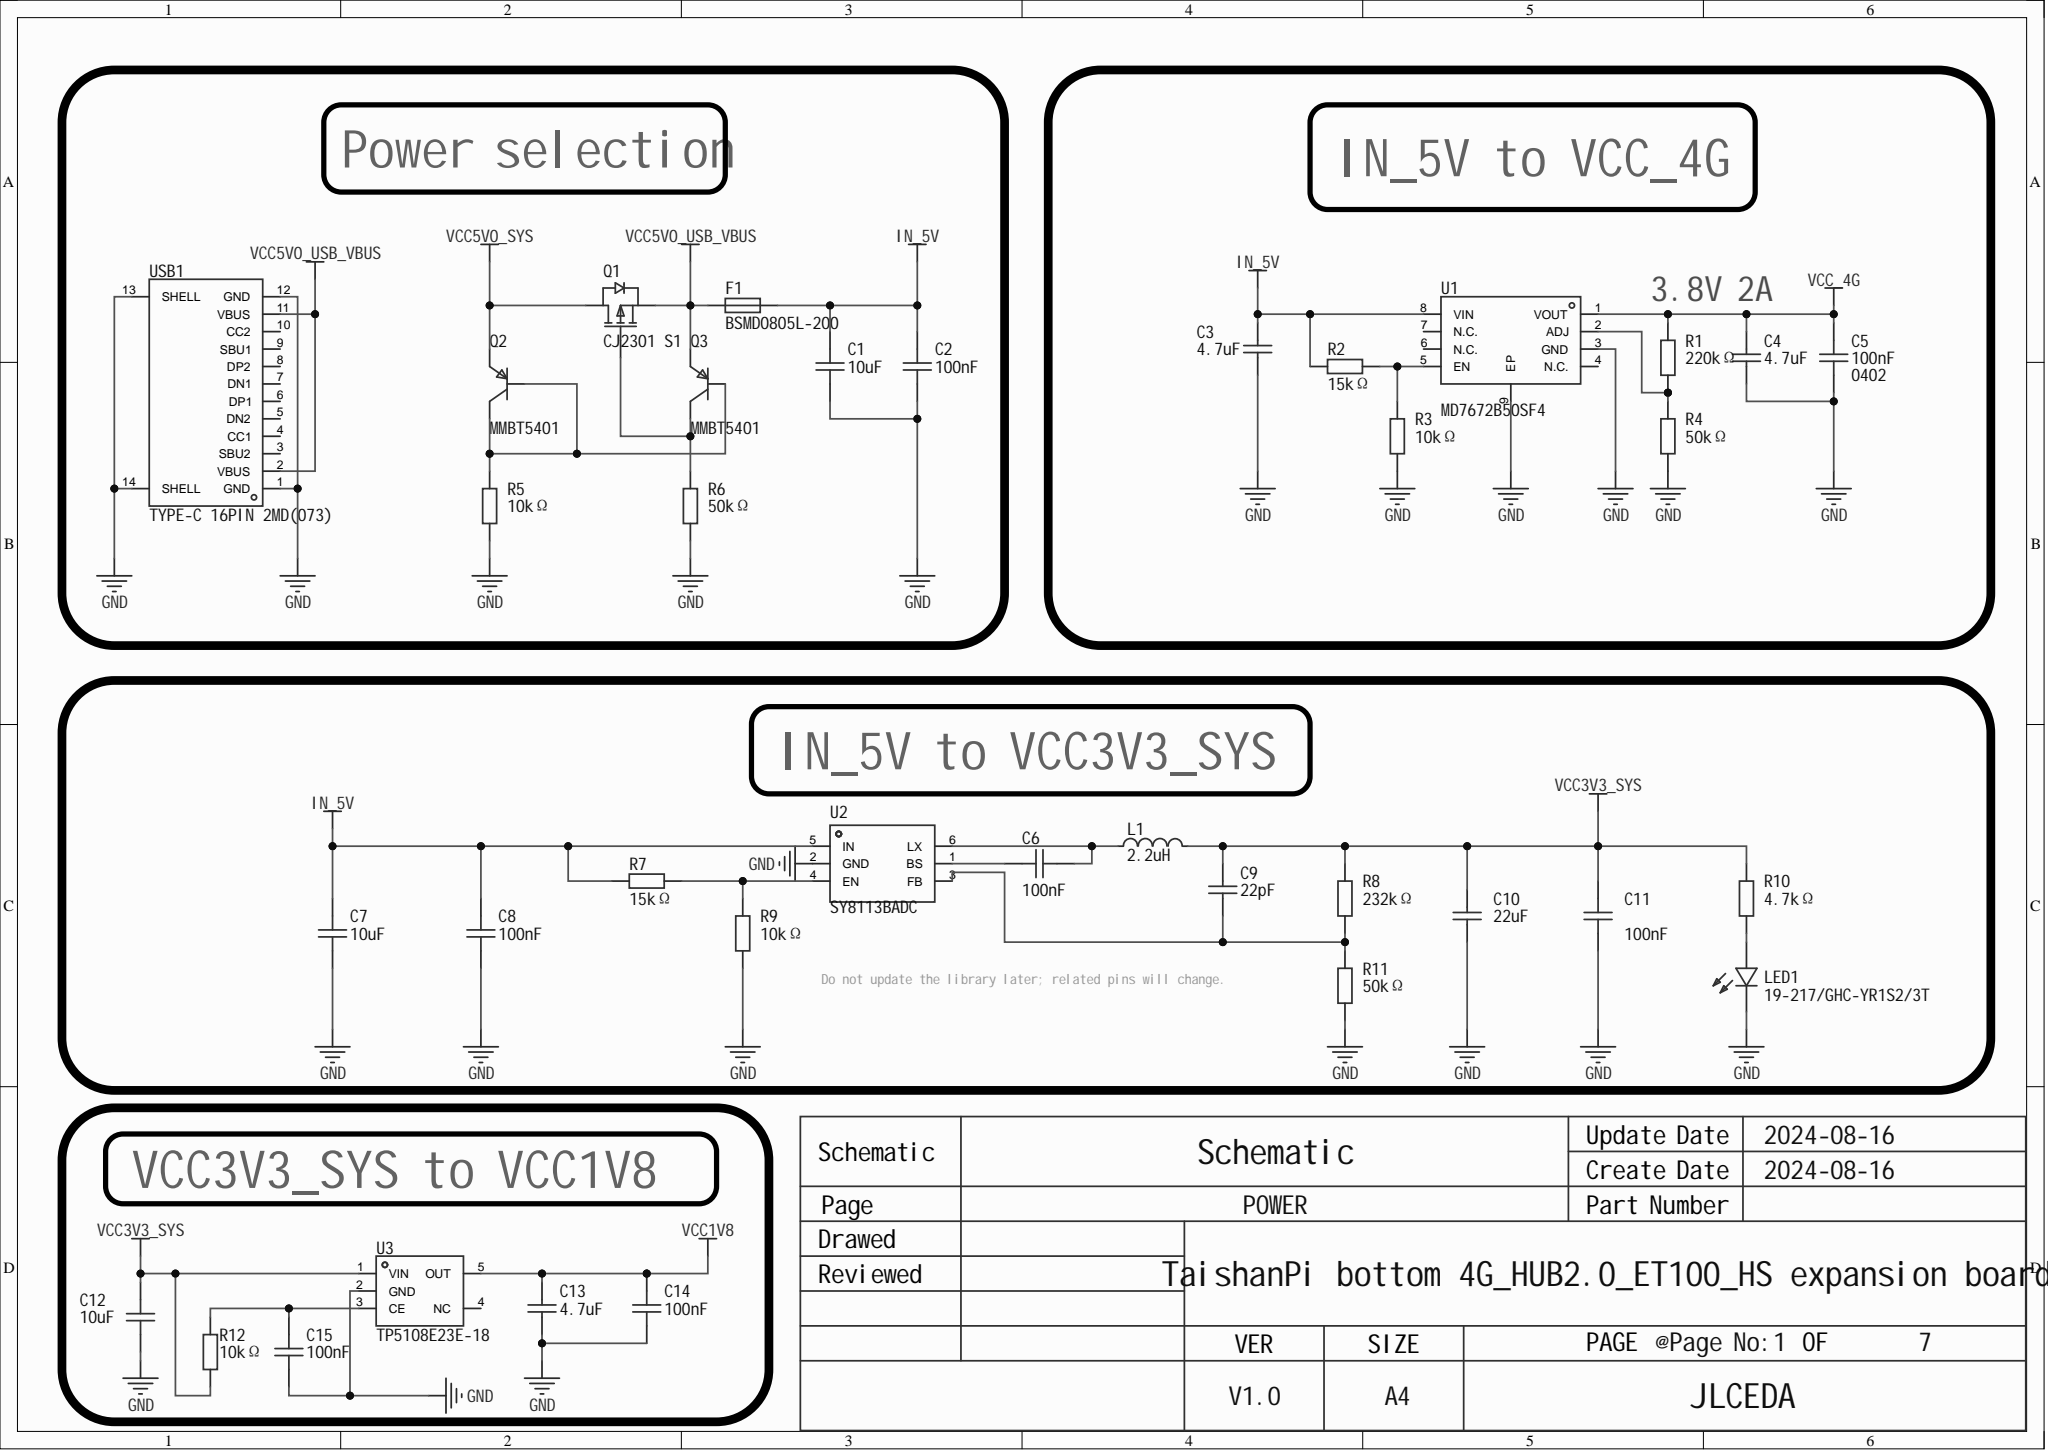Circuit board | Altium Designer | 209 parts | 149 nets | one sheet of the schematic
Parts on this sheet (reference | value | footprint):
C1 | 10uF | r0603
C2 | 100nF | r0603
C3 | 4.7uF | C0603
C4 | 4.7uF | C0603
C7 | 10uF | r0603
C8 | 100nF | r0603
C9 | 22pF | R0402
C10 | 22uF | r0603
C11 | 100nF | r0603
C12 | 10uF | r0603
C13 | 4.7uF | r0603
C14 | 100nF | C0603
C15 | 100nF | C0603
F1 | BSMD0805L-200 | F0805
L1 | 2.2uH | IND-SMD_L2.5-W2.0_WPN252012H
LED1 | 19-217/GHC-YR1S2/3T | LED0603-RD
Q1 | CJ2301 S1 | SOT-23-3_L3.0-W1.7-P0.95-LS2.9-BR
Q2 | MMBT5401 | SOT-23-3_L2.9-W1.3-P1.90-LS2.4-BR
Q3 | MMBT5401 | SOT-23-3_L2.9-W1.3-P1.90-LS2.4-BR
R1 | 220kΩ | R0402
R2 | 15kΩ | R0402
R3 | 10kΩ | R0402
R4 | 50kΩ | R0402
R5 | 10kΩ | R0402
R6 | 50kΩ | R0402
R7 | 15kΩ | R0402
R8 | 232kΩ | R0402
R9 | 10kΩ | R0402
R10 | 4.7kΩ | R0402
R11 | 50kΩ | R0402
R12 | 10kΩ | R0603
U1 | MD7672B50SF4 | ESOP-8_L4.9-W3.9-P1.27-LS6.0-BL-EP
U2 | SY8113BADC | TSOT-23-6_L2.9-W1.6-P0.95-LS2.8-BR
U3 | TP5108E23E-18 | SOT-23-5_L3.0-W1.7-P0.95-LS2.8-BL
USB1 | TYPE-C 16PIN 2MD(073) | USB-C-SMD_TYPE-C-6PIN-2MD-073
Nets of these parts (net: part-pin ...):
VCC_4G: C4-2 R1-2 U1-1
VCC5V0_USB_VBUS: F1-1 Q1-2 Q3-2 USB1-2 USB1-11
VCC5V0_SYS: Q1-3 Q2-2
VCC3V3_SYS: C9-2 C10-2 C11-2 C12-2 L1-2 R8-2 R10-2 R12-1 U3-1
VCC1V8: C13-2 C14-2 U3-5
NetR7_1: R7-1 R9-2 U2-4
NetR2_1: R2-1 R3-2 U1-5
NetR1_1: R1-1 R4-2 U1-2
NetQ2_1: Q2-1 Q2-3 Q3-1 R5-2
NetQ1_1: Q1-1 Q3-3 R6-2
NetLED1_2: LED1-2 R10-1
NetC15_2: C15-2 R12-2 U3-3
NetC9_1: C9-1 R8-1 R11-2 U2-3
NetC6_2: U2-1
NetC6_1: L1-1 U2-6
IN_5V: C1-2 C2-2 C3-2 C7-2 C8-2 F1-2 R2-2 R7-2 U1-8 U2-5
GND: C1-1 C2-1 C3-1 C4-1 C7-1 C8-1 C10-1 C11-1 C12-1 C13-1 C14-1 C15-1 LED1-1 R3-1 R4-1 R5-1 R6-1 R9-1 R11-1 U1-3 U1-9 U2-2 U3-2 USB1-1 USB1-12 USB1-13 USB1-14